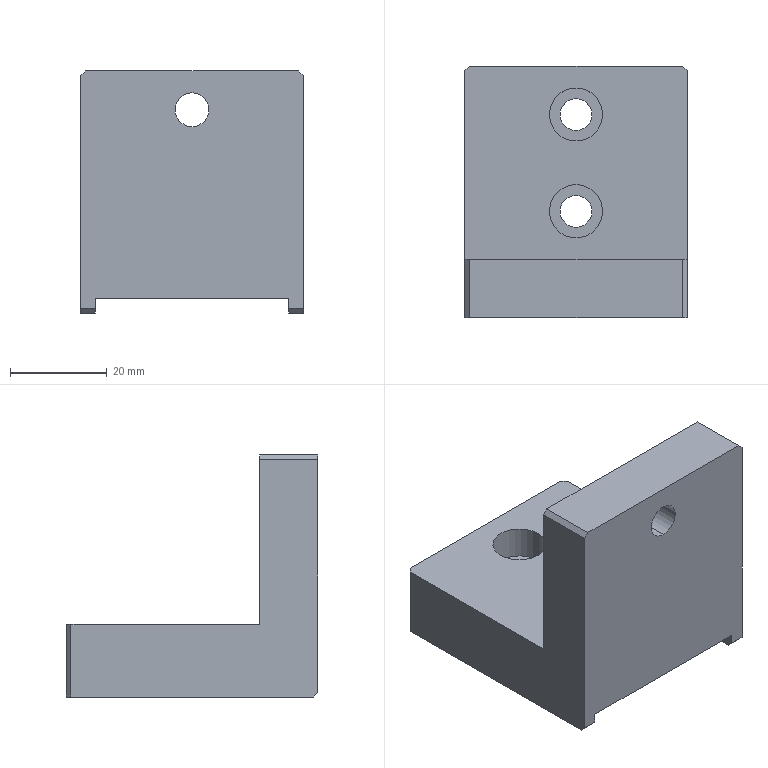Part | SolidWorks | features HoleWzd 2, ICE 2, Chamfer 1, Extrusion 1 | 1 solid | 30 faces | box 46 x 52 x 50 mm | volume 46820 mm3 | plane 20 | cylinder 10 | commonest cylinder face diameters 6.6 x4 11 x4 7 x2
STEP:
#1=CARTESIAN_POINT('',(0.,-6.,13.5));
#2=VERTEX_POINT('',#1);
#3=CARTESIAN_POINT('',(0.,-6.,20.5));
#4=VERTEX_POINT('',#3);
#5=CARTESIAN_POINT('',(0.,-6.,17.));
#6=DIRECTION('',(0.,1.,0.));
#7=DIRECTION('',(0.,0.,1.));
#8=AXIS2_PLACEMENT_3D('',#5,#6,#7);
#9=CIRCLE('',#8,3.5);
#10=EDGE_CURVE('',#2,#4,#9,.T.);
#11=ORIENTED_EDGE('',*,*,#10,.F.);
#12=CARTESIAN_POINT('',(0.,6.,13.5));
#13=VERTEX_POINT('',#12);
#14=CARTESIAN_POINT('',(0.,6.,13.5));
#15=DIRECTION('',(0.,1.,0.));
#16=VECTOR('',#15,1000.);
#17=LINE('',#14,#16);
#18=EDGE_CURVE('',#2,#13,#17,.T.);
#19=ORIENTED_EDGE('',*,*,#18,.T.);
#20=CARTESIAN_POINT('',(0.,6.,20.5));
#21=VERTEX_POINT('',#20);
#22=CARTESIAN_POINT('',(0.,6.,17.));
#23=DIRECTION('',(0.,1.,0.));
#24=DIRECTION('',(0.,0.,1.));
#25=AXIS2_PLACEMENT_3D('',#22,#23,#24);
#26=CIRCLE('',#25,3.5);
#27=EDGE_CURVE('',#13,#21,#26,.T.);
#28=ORIENTED_EDGE('',*,*,#27,.T.);
#29=CARTESIAN_POINT('',(0.,6.,20.5));
#30=DIRECTION('',(0.,1.,0.));
#31=VECTOR('',#30,1000.);
#32=LINE('',#29,#31);
#33=EDGE_CURVE('',#4,#21,#32,.T.);
#34=ORIENTED_EDGE('',*,*,#33,.F.);
#35=EDGE_LOOP('',(#11,#19,#28,#34));
#36=FACE_OUTER_BOUND('',#35,.T.);
#37=CARTESIAN_POINT('',(0.,6.,17.));
#38=DIRECTION('',(0.,1.,0.));
#39=DIRECTION('',(0.,0.,1.));
#40=AXIS2_PLACEMENT_3D('',#37,#38,#39);
#41=CYLINDRICAL_SURFACE('',#40,3.5);
#42=ADVANCED_FACE('',(#36),#41,.F.);
#43=CARTESIAN_POINT('',(-5.5,16.,-16.8));
#44=VERTEX_POINT('',#43);
#45=CARTESIAN_POINT('',(5.5,16.,-16.8));
#46=VERTEX_POINT('',#45);
#47=CARTESIAN_POINT('',(0.,16.,-16.8));
#48=DIRECTION('',(0.,0.,1.));
#49=DIRECTION('',(1.,0.,0.));
#50=AXIS2_PLACEMENT_3D('',#47,#48,#49);
#51=CIRCLE('',#50,5.5);
#52=EDGE_CURVE('',#44,#46,#51,.T.);
#53=ORIENTED_EDGE('',*,*,#52,.F.);
#54=CARTESIAN_POINT('',(-5.5,16.,-10.));
#55=VERTEX_POINT('',#54);
#56=CARTESIAN_POINT('',(-5.5,16.,-10.));
#57=DIRECTION('',(0.,0.,1.));
#58=VECTOR('',#57,1000.);
#59=LINE('',#56,#58);
#60=EDGE_CURVE('',#44,#55,#59,.T.);
#61=ORIENTED_EDGE('',*,*,#60,.T.);
#62=CARTESIAN_POINT('',(5.5,16.,-10.));
#63=VERTEX_POINT('',#62);
#64=CARTESIAN_POINT('',(0.,16.,-10.));
#65=DIRECTION('',(0.,0.,1.));
#66=DIRECTION('',(1.,0.,0.));
#67=AXIS2_PLACEMENT_3D('',#64,#65,#66);
#68=CIRCLE('',#67,5.5);
#69=EDGE_CURVE('',#55,#63,#68,.T.);
#70=ORIENTED_EDGE('',*,*,#69,.T.);
#71=CARTESIAN_POINT('',(5.5,16.,-10.));
#72=DIRECTION('',(0.,0.,1.));
#73=VECTOR('',#72,1000.);
#74=LINE('',#71,#73);
#75=EDGE_CURVE('',#46,#63,#74,.T.);
#76=ORIENTED_EDGE('',*,*,#75,.F.);
#77=EDGE_LOOP('',(#53,#61,#70,#76));
#78=FACE_OUTER_BOUND('',#77,.T.);
#79=CARTESIAN_POINT('',(0.,16.,-10.));
#80=DIRECTION('',(0.,0.,1.));
#81=DIRECTION('',(1.,0.,0.));
#82=AXIS2_PLACEMENT_3D('',#79,#80,#81);
#83=CYLINDRICAL_SURFACE('',#82,5.5);
#84=ADVANCED_FACE('',(#78),#83,.F.);
#85=CARTESIAN_POINT('',(3.3,16.,-22.));
#86=VERTEX_POINT('',#85);
#87=CARTESIAN_POINT('',(-3.3,16.,-22.));
#88=VERTEX_POINT('',#87);
#89=CARTESIAN_POINT('',(0.,16.,-22.));
#90=DIRECTION('',(0.,0.,-1.));
#91=DIRECTION('',(-1.,0.,0.));
#92=AXIS2_PLACEMENT_3D('',#89,#90,#91);
#93=CIRCLE('',#92,3.3);
#94=EDGE_CURVE('',#86,#88,#93,.T.);
#95=ORIENTED_EDGE('',*,*,#94,.T.);
#96=CARTESIAN_POINT('',(-3.3,16.,-16.8));
#97=VERTEX_POINT('',#96);
#98=CARTESIAN_POINT('',(-3.3,16.,-10.));
#99=DIRECTION('',(0.,0.,1.));
#100=VECTOR('',#99,1000.);
#101=LINE('',#98,#100);
#102=EDGE_CURVE('',#88,#97,#101,.T.);
#103=ORIENTED_EDGE('',*,*,#102,.T.);
#104=CARTESIAN_POINT('',(3.3,16.,-16.8));
#105=VERTEX_POINT('',#104);
#106=CARTESIAN_POINT('',(0.,16.,-16.8));
#107=DIRECTION('',(0.,0.,1.));
#108=DIRECTION('',(1.,0.,0.));
#109=AXIS2_PLACEMENT_3D('',#106,#107,#108);
#110=CIRCLE('',#109,3.3);
#111=EDGE_CURVE('',#97,#105,#110,.T.);
#112=ORIENTED_EDGE('',*,*,#111,.T.);
#113=CARTESIAN_POINT('',(3.3,16.,-10.));
#114=DIRECTION('',(0.,0.,1.));
#115=VECTOR('',#114,1000.);
#116=LINE('',#113,#115);
#117=EDGE_CURVE('',#86,#105,#116,.T.);
#118=ORIENTED_EDGE('',*,*,#117,.F.);
#119=EDGE_LOOP('',(#95,#103,#112,#118));
#120=FACE_OUTER_BOUND('',#119,.T.);
#121=CARTESIAN_POINT('',(0.,16.,-10.));
#122=DIRECTION('',(0.,0.,1.));
#123=DIRECTION('',(1.,0.,0.));
#124=AXIS2_PLACEMENT_3D('',#121,#122,#123);
#125=CYLINDRICAL_SURFACE('',#124,3.3);
#126=ADVANCED_FACE('',(#120),#125,.F.);
#127=CARTESIAN_POINT('',(-5.5,36.,-16.8));
#128=VERTEX_POINT('',#127);
#129=CARTESIAN_POINT('',(5.5,36.,-16.8));
#130=VERTEX_POINT('',#129);
#131=CARTESIAN_POINT('',(0.,36.,-16.8));
#132=DIRECTION('',(0.,0.,1.));
#133=DIRECTION('',(1.,0.,0.));
#134=AXIS2_PLACEMENT_3D('',#131,#132,#133);
#135=CIRCLE('',#134,5.5);
#136=EDGE_CURVE('',#128,#130,#135,.T.);
#137=ORIENTED_EDGE('',*,*,#136,.F.);
#138=CARTESIAN_POINT('',(-5.5,36.,-10.));
#139=VERTEX_POINT('',#138);
#140=CARTESIAN_POINT('',(-5.5,36.,-10.));
#141=DIRECTION('',(0.,0.,1.));
#142=VECTOR('',#141,1000.);
#143=LINE('',#140,#142);
#144=EDGE_CURVE('',#128,#139,#143,.T.);
#145=ORIENTED_EDGE('',*,*,#144,.T.);
#146=CARTESIAN_POINT('',(5.5,36.,-10.));
#147=VERTEX_POINT('',#146);
#148=CARTESIAN_POINT('',(0.,36.,-10.));
#149=DIRECTION('',(0.,0.,1.));
#150=DIRECTION('',(1.,0.,0.));
#151=AXIS2_PLACEMENT_3D('',#148,#149,#150);
#152=CIRCLE('',#151,5.5);
#153=EDGE_CURVE('',#139,#147,#152,.T.);
#154=ORIENTED_EDGE('',*,*,#153,.T.);
#155=CARTESIAN_POINT('',(5.5,36.,-10.));
#156=DIRECTION('',(0.,0.,1.));
#157=VECTOR('',#156,1000.);
#158=LINE('',#155,#157);
#159=EDGE_CURVE('',#130,#147,#158,.T.);
#160=ORIENTED_EDGE('',*,*,#159,.F.);
#161=EDGE_LOOP('',(#137,#145,#154,#160));
#162=FACE_OUTER_BOUND('',#161,.T.);
#163=CARTESIAN_POINT('',(0.,36.,-10.));
#164=DIRECTION('',(0.,0.,1.));
#165=DIRECTION('',(1.,0.,0.));
#166=AXIS2_PLACEMENT_3D('',#163,#164,#165);
#167=CYLINDRICAL_SURFACE('',#166,5.5);
#168=ADVANCED_FACE('',(#162),#167,.F.);
#169=CARTESIAN_POINT('',(3.3,36.,-22.));
#170=VERTEX_POINT('',#169);
#171=CARTESIAN_POINT('',(-3.3,36.,-22.));
#172=VERTEX_POINT('',#171);
#173=CARTESIAN_POINT('',(0.,36.,-22.));
#174=DIRECTION('',(0.,0.,-1.));
#175=DIRECTION('',(-1.,0.,0.));
#176=AXIS2_PLACEMENT_3D('',#173,#174,#175);
#177=CIRCLE('',#176,3.3);
#178=EDGE_CURVE('',#170,#172,#177,.T.);
#179=ORIENTED_EDGE('',*,*,#178,.T.);
#180=CARTESIAN_POINT('',(-3.3,36.,-16.8));
#181=VERTEX_POINT('',#180);
#182=CARTESIAN_POINT('',(-3.3,36.,-10.));
#183=DIRECTION('',(0.,0.,1.));
#184=VECTOR('',#183,1000.);
#185=LINE('',#182,#184);
#186=EDGE_CURVE('',#172,#181,#185,.T.);
#187=ORIENTED_EDGE('',*,*,#186,.T.);
#188=CARTESIAN_POINT('',(3.3,36.,-16.8));
#189=VERTEX_POINT('',#188);
#190=CARTESIAN_POINT('',(0.,36.,-16.8));
#191=DIRECTION('',(0.,0.,1.));
#192=DIRECTION('',(1.,0.,0.));
#193=AXIS2_PLACEMENT_3D('',#190,#191,#192);
#194=CIRCLE('',#193,3.3);
#195=EDGE_CURVE('',#181,#189,#194,.T.);
#196=ORIENTED_EDGE('',*,*,#195,.T.);
#197=CARTESIAN_POINT('',(3.3,36.,-10.));
#198=DIRECTION('',(0.,0.,1.));
#199=VECTOR('',#198,1000.);
#200=LINE('',#197,#199);
#201=EDGE_CURVE('',#170,#189,#200,.T.);
#202=ORIENTED_EDGE('',*,*,#201,.F.);
#203=EDGE_LOOP('',(#179,#187,#196,#202));
#204=FACE_OUTER_BOUND('',#203,.T.);
#205=CARTESIAN_POINT('',(0.,36.,-10.));
#206=DIRECTION('',(0.,0.,1.));
#207=DIRECTION('',(1.,0.,0.));
#208=AXIS2_PLACEMENT_3D('',#205,#206,#207);
#209=CYLINDRICAL_SURFACE('',#208,3.3);
#210=ADVANCED_FACE('',(#204),#209,.F.);
#211=CARTESIAN_POINT('',(-22.,6.,25.));
#212=VERTEX_POINT('',#211);
#213=CARTESIAN_POINT('',(22.,6.,25.));
#214=VERTEX_POINT('',#213);
#215=CARTESIAN_POINT('',(-23.,6.,25.));
#216=DIRECTION('',(1.,0.,0.));
#217=VECTOR('',#216,1000.);
#218=LINE('',#215,#217);
#219=EDGE_CURVE('',#212,#214,#218,.T.);
#220=ORIENTED_EDGE('',*,*,#219,.T.);
#221=CARTESIAN_POINT('',(23.,6.,24.));
#222=VERTEX_POINT('',#221);
#223=CARTESIAN_POINT('',(23.,6.,24.));
#224=DIRECTION('',(0.7071,0.,-0.7071));
#225=VECTOR('',#224,1000.);
#226=LINE('',#223,#225);
#227=EDGE_CURVE('',#214,#222,#226,.T.);
#228=ORIENTED_EDGE('',*,*,#227,.T.);
#229=CARTESIAN_POINT('',(23.,6.,-10.));
#230=VERTEX_POINT('',#229);
#231=CARTESIAN_POINT('',(23.,6.,25.));
#232=DIRECTION('',(0.,0.,-1.));
#233=VECTOR('',#232,1000.);
#234=LINE('',#231,#233);
#235=EDGE_CURVE('',#222,#230,#234,.T.);
#236=ORIENTED_EDGE('',*,*,#235,.T.);
#237=CARTESIAN_POINT('',(-23.,6.,-10.));
#238=VERTEX_POINT('',#237);
#239=CARTESIAN_POINT('',(23.,6.,-10.));
#240=DIRECTION('',(1.,0.,0.));
#241=VECTOR('',#240,1000.);
#242=LINE('',#239,#241);
#243=EDGE_CURVE('',#238,#230,#242,.T.);
#244=ORIENTED_EDGE('',*,*,#243,.F.);
#245=CARTESIAN_POINT('',(-23.,6.,24.));
#246=VERTEX_POINT('',#245);
#247=CARTESIAN_POINT('',(-23.,6.,25.));
#248=DIRECTION('',(0.,0.,1.));
#249=VECTOR('',#248,1000.);
#250=LINE('',#247,#249);
#251=EDGE_CURVE('',#238,#246,#250,.T.);
#252=ORIENTED_EDGE('',*,*,#251,.T.);
#253=CARTESIAN_POINT('',(-22.,6.,25.));
#254=DIRECTION('',(0.7071,0.,0.7071));
#255=VECTOR('',#254,1000.);
#256=LINE('',#253,#255);
#257=EDGE_CURVE('',#246,#212,#256,.T.);
#258=ORIENTED_EDGE('',*,*,#257,.T.);
#259=EDGE_LOOP('',(#220,#228,#236,#244,#252,#258));
#260=FACE_OUTER_BOUND('',#259,.T.);
#261=CARTESIAN_POINT('',(0.,6.,17.));
#262=DIRECTION('',(0.,1.,0.));
#263=DIRECTION('',(0.,0.,1.));
#264=AXIS2_PLACEMENT_3D('',#261,#262,#263);
#265=CIRCLE('',#264,3.5);
#266=EDGE_CURVE('',#21,#13,#265,.T.);
#267=ORIENTED_EDGE('',*,*,#266,.F.);
#268=ORIENTED_EDGE('',*,*,#27,.F.);
#269=EDGE_LOOP('',(#267,#268));
#270=FACE_BOUND('',#269,.T.);
#271=CARTESIAN_POINT('',(0.,6.,0.));
#272=DIRECTION('',(0.,-1.,0.));
#273=DIRECTION('',(0.,0.,-1.));
#274=AXIS2_PLACEMENT_3D('',#271,#272,#273);
#275=PLANE('',#274);
#276=ADVANCED_FACE('',(#260,#270),#275,.F.);
#277=CARTESIAN_POINT('',(23.,45.,-25.));
#278=VERTEX_POINT('',#277);
#279=CARTESIAN_POINT('',(23.,-5.,-25.));
#280=VERTEX_POINT('',#279);
#281=CARTESIAN_POINT('',(23.,6.,-25.));
#282=DIRECTION('',(0.,-1.,0.));
#283=VECTOR('',#282,1000.);
#284=LINE('',#281,#283);
#285=EDGE_CURVE('',#278,#280,#284,.T.);
#286=ORIENTED_EDGE('',*,*,#285,.T.);
#287=CARTESIAN_POINT('',(20.,-5.,-25.));
#288=VERTEX_POINT('',#287);
#289=CARTESIAN_POINT('',(20.,-5.,-25.));
#290=DIRECTION('',(-1.,0.,0.));
#291=VECTOR('',#290,1000.);
#292=LINE('',#289,#291);
#293=EDGE_CURVE('',#280,#288,#292,.T.);
#294=ORIENTED_EDGE('',*,*,#293,.T.);
#295=CARTESIAN_POINT('',(20.,46.,-25.));
#296=VERTEX_POINT('',#295);
#297=CARTESIAN_POINT('',(20.,46.,-25.));
#298=DIRECTION('',(0.,-1.,0.));
#299=VECTOR('',#298,1000.);
#300=LINE('',#297,#299);
#301=EDGE_CURVE('',#296,#288,#300,.T.);
#302=ORIENTED_EDGE('',*,*,#301,.F.);
#303=CARTESIAN_POINT('',(22.,46.,-25.));
#304=VERTEX_POINT('',#303);
#305=CARTESIAN_POINT('',(23.,46.,-25.));
#306=DIRECTION('',(-1.,0.,0.));
#307=VECTOR('',#306,1000.);
#308=LINE('',#305,#307);
#309=EDGE_CURVE('',#304,#296,#308,.T.);
#310=ORIENTED_EDGE('',*,*,#309,.F.);
#311=CARTESIAN_POINT('',(22.,46.,-25.));
#312=DIRECTION('',(0.7071,-0.7071,0.));
#313=VECTOR('',#312,1000.);
#314=LINE('',#311,#313);
#315=EDGE_CURVE('',#304,#278,#314,.T.);
#316=ORIENTED_EDGE('',*,*,#315,.T.);
#317=EDGE_LOOP('',(#286,#294,#302,#310,#316));
#318=FACE_OUTER_BOUND('',#317,.T.);
#319=CARTESIAN_POINT('',(-23.,6.,-25.));
#320=DIRECTION('',(0.,0.,1.));
#321=DIRECTION('',(1.,0.,0.));
#322=AXIS2_PLACEMENT_3D('',#319,#320,#321);
#323=PLANE('',#322);
#324=ADVANCED_FACE('',(#318),#323,.F.);
#325=CARTESIAN_POINT('',(23.,-6.,24.));
#326=VERTEX_POINT('',#325);
#327=CARTESIAN_POINT('',(23.,-6.,-24.));
#328=VERTEX_POINT('',#327);
#329=CARTESIAN_POINT('',(23.,-6.,25.));
#330=DIRECTION('',(0.,0.,-1.));
#331=VECTOR('',#330,1000.);
#332=LINE('',#329,#331);
#333=EDGE_CURVE('',#326,#328,#332,.T.);
#334=ORIENTED_EDGE('',*,*,#333,.T.);
#335=CARTESIAN_POINT('',(23.,-5.,-25.));
#336=DIRECTION('',(0.,0.7071,-0.7071));
#337=VECTOR('',#336,1000.);
#338=LINE('',#335,#337);
#339=EDGE_CURVE('',#328,#280,#338,.T.);
#340=ORIENTED_EDGE('',*,*,#339,.T.);
#341=ORIENTED_EDGE('',*,*,#285,.F.);
#342=CARTESIAN_POINT('',(23.,45.,-10.));
#343=VERTEX_POINT('',#342);
#344=CARTESIAN_POINT('',(23.,45.,25.));
#345=DIRECTION('',(0.,0.,1.));
#346=VECTOR('',#345,1000.);
#347=LINE('',#344,#346);
#348=EDGE_CURVE('',#278,#343,#347,.T.);
#349=ORIENTED_EDGE('',*,*,#348,.T.);
#350=CARTESIAN_POINT('',(23.,46.,-10.));
#351=DIRECTION('',(0.,-1.,0.));
#352=VECTOR('',#351,1000.);
#353=LINE('',#350,#352);
#354=EDGE_CURVE('',#343,#230,#353,.T.);
#355=ORIENTED_EDGE('',*,*,#354,.T.);
#356=ORIENTED_EDGE('',*,*,#235,.F.);
#357=CARTESIAN_POINT('',(23.,6.,24.));
#358=DIRECTION('',(0.,-1.,0.));
#359=VECTOR('',#358,1000.);
#360=LINE('',#357,#359);
#361=EDGE_CURVE('',#222,#326,#360,.T.);
#362=ORIENTED_EDGE('',*,*,#361,.T.);
#363=EDGE_LOOP('',(#334,#340,#341,#349,#355,#356,#362));
#364=FACE_OUTER_BOUND('',#363,.T.);
#365=CARTESIAN_POINT('',(23.,6.,25.));
#366=DIRECTION('',(-1.,0.,0.));
#367=DIRECTION('',(0.,0.,1.));
#368=AXIS2_PLACEMENT_3D('',#365,#366,#367);
#369=PLANE('',#368);
#370=ADVANCED_FACE('',(#364),#369,.F.);
#371=CARTESIAN_POINT('',(-20.,-5.,-25.));
#372=VERTEX_POINT('',#371);
#373=CARTESIAN_POINT('',(-20.,46.,-25.));
#374=VERTEX_POINT('',#373);
#375=CARTESIAN_POINT('',(-20.,46.,-25.));
#376=DIRECTION('',(0.,1.,0.));
#377=VECTOR('',#376,1000.);
#378=LINE('',#375,#377);
#379=EDGE_CURVE('',#372,#374,#378,.T.);
#380=ORIENTED_EDGE('',*,*,#379,.F.);
#381=CARTESIAN_POINT('',(-23.,-5.,-25.));
#382=VERTEX_POINT('',#381);
#383=CARTESIAN_POINT('',(-23.,-5.,-25.));
#384=DIRECTION('',(-1.,0.,0.));
#385=VECTOR('',#384,1000.);
#386=LINE('',#383,#385);
#387=EDGE_CURVE('',#372,#382,#386,.T.);
#388=ORIENTED_EDGE('',*,*,#387,.T.);
#389=CARTESIAN_POINT('',(-23.,45.,-25.));
#390=VERTEX_POINT('',#389);
#391=CARTESIAN_POINT('',(-23.,6.,-25.));
#392=DIRECTION('',(0.,-1.,0.));
#393=VECTOR('',#392,1000.);
#394=LINE('',#391,#393);
#395=EDGE_CURVE('',#390,#382,#394,.T.);
#396=ORIENTED_EDGE('',*,*,#395,.F.);
#397=CARTESIAN_POINT('',(-22.,46.,-25.));
#398=VERTEX_POINT('',#397);
#399=CARTESIAN_POINT('',(-22.,46.,-25.));
#400=DIRECTION('',(0.7071,0.7071,0.));
#401=VECTOR('',#400,1000.);
#402=LINE('',#399,#401);
#403=EDGE_CURVE('',#390,#398,#402,.T.);
#404=ORIENTED_EDGE('',*,*,#403,.T.);
#405=CARTESIAN_POINT('',(23.,46.,-25.));
#406=DIRECTION('',(-1.,0.,0.));
#407=VECTOR('',#406,1000.);
#408=LINE('',#405,#407);
#409=EDGE_CURVE('',#374,#398,#408,.T.);
#410=ORIENTED_EDGE('',*,*,#409,.F.);
#411=EDGE_LOOP('',(#380,#388,#396,#404,#410));
#412=FACE_OUTER_BOUND('',#411,.T.);
#413=CARTESIAN_POINT('',(-23.,6.,-25.));
#414=DIRECTION('',(0.,0.,1.));
#415=DIRECTION('',(1.,0.,0.));
#416=AXIS2_PLACEMENT_3D('',#413,#414,#415);
#417=PLANE('',#416);
#418=ADVANCED_FACE('',(#412),#417,.F.);
#419=ORIENTED_EDGE('',*,*,#395,.T.);
#420=CARTESIAN_POINT('',(-23.,-6.,-24.));
#421=VERTEX_POINT('',#420);
#422=CARTESIAN_POINT('',(-23.,-5.,-25.));
#423=DIRECTION('',(0.,-0.7071,0.7071));
#424=VECTOR('',#423,1000.);
#425=LINE('',#422,#424);
#426=EDGE_CURVE('',#382,#421,#425,.T.);
#427=ORIENTED_EDGE('',*,*,#426,.T.);
#428=CARTESIAN_POINT('',(-23.,-6.,24.));
#429=VERTEX_POINT('',#428);
#430=CARTESIAN_POINT('',(-23.,-6.,25.));
#431=DIRECTION('',(0.,0.,1.));
#432=VECTOR('',#431,1000.);
#433=LINE('',#430,#432);
#434=EDGE_CURVE('',#421,#429,#433,.T.);
#435=ORIENTED_EDGE('',*,*,#434,.T.);
#436=CARTESIAN_POINT('',(-23.,6.,24.));
#437=DIRECTION('',(0.,1.,0.));
#438=VECTOR('',#437,1000.);
#439=LINE('',#436,#438);
#440=EDGE_CURVE('',#429,#246,#439,.T.);
#441=ORIENTED_EDGE('',*,*,#440,.T.);
#442=ORIENTED_EDGE('',*,*,#251,.F.);
#443=CARTESIAN_POINT('',(-23.,45.,-10.));
#444=VERTEX_POINT('',#443);
#445=CARTESIAN_POINT('',(-23.,46.,-10.));
#446=DIRECTION('',(0.,-1.,0.));
#447=VECTOR('',#446,1000.);
#448=LINE('',#445,#447);
#449=EDGE_CURVE('',#444,#238,#448,.T.);
#450=ORIENTED_EDGE('',*,*,#449,.F.);
#451=CARTESIAN_POINT('',(-23.,45.,25.));
#452=DIRECTION('',(0.,0.,-1.));
#453=VECTOR('',#452,1000.);
#454=LINE('',#451,#453);
#455=EDGE_CURVE('',#444,#390,#454,.T.);
#456=ORIENTED_EDGE('',*,*,#455,.T.);
#457=EDGE_LOOP('',(#419,#427,#435,#441,#442,#450,#456));
#458=FACE_OUTER_BOUND('',#457,.T.);
#459=CARTESIAN_POINT('',(-23.,6.,25.));
#460=DIRECTION('',(1.,0.,0.));
#461=DIRECTION('',(0.,0.,-1.));
#462=AXIS2_PLACEMENT_3D('',#459,#460,#461);
#463=PLANE('',#462);
#464=ADVANCED_FACE('',(#458),#463,.F.);
#465=CARTESIAN_POINT('',(-22.,-6.,25.));
#466=VERTEX_POINT('',#465);
#467=CARTESIAN_POINT('',(22.,-6.,25.));
#468=VERTEX_POINT('',#467);
#469=CARTESIAN_POINT('',(-23.,-6.,25.));
#470=DIRECTION('',(1.,0.,0.));
#471=VECTOR('',#470,1000.);
#472=LINE('',#469,#471);
#473=EDGE_CURVE('',#466,#468,#472,.T.);
#474=ORIENTED_EDGE('',*,*,#473,.T.);
#475=CARTESIAN_POINT('',(22.,6.,25.));
#476=DIRECTION('',(0.,1.,0.));
#477=VECTOR('',#476,1000.);
#478=LINE('',#475,#477);
#479=EDGE_CURVE('',#468,#214,#478,.T.);
#480=ORIENTED_EDGE('',*,*,#479,.T.);
#481=ORIENTED_EDGE('',*,*,#219,.F.);
#482=CARTESIAN_POINT('',(-22.,6.,25.));
#483=DIRECTION('',(0.,-1.,0.));
#484=VECTOR('',#483,1000.);
#485=LINE('',#482,#484);
#486=EDGE_CURVE('',#212,#466,#485,.T.);
#487=ORIENTED_EDGE('',*,*,#486,.T.);
#488=EDGE_LOOP('',(#474,#480,#481,#487));
#489=FACE_OUTER_BOUND('',#488,.T.);
#490=CARTESIAN_POINT('',(-23.,6.,25.));
#491=DIRECTION('',(0.,0.,-1.));
#492=DIRECTION('',(-1.,0.,0.));
#493=AXIS2_PLACEMENT_3D('',#490,#491,#492);
#494=PLANE('',#493);
#495=ADVANCED_FACE('',(#489),#494,.F.);
#496=CARTESIAN_POINT('',(0.,-6.,17.));
#497=DIRECTION('',(0.,1.,0.));
#498=DIRECTION('',(0.,0.,1.));
#499=AXIS2_PLACEMENT_3D('',#496,#497,#498);
#500=CIRCLE('',#499,3.5);
#501=EDGE_CURVE('',#4,#2,#500,.T.);
#502=ORIENTED_EDGE('',*,*,#501,.T.);
#503=ORIENTED_EDGE('',*,*,#10,.T.);
#504=EDGE_LOOP('',(#502,#503));
#505=FACE_BOUND('',#504,.T.);
#506=CARTESIAN_POINT('',(20.,-6.,-22.));
#507=VERTEX_POINT('',#506);
#508=CARTESIAN_POINT('',(20.,-6.,-24.));
#509=VERTEX_POINT('',#508);
#510=CARTESIAN_POINT('',(20.,-6.,-22.));
#511=DIRECTION('',(0.,0.,-1.));
#512=VECTOR('',#511,1000.);
#513=LINE('',#510,#512);
#514=EDGE_CURVE('',#507,#509,#513,.T.);
#515=ORIENTED_EDGE('',*,*,#514,.T.);
#516=CARTESIAN_POINT('',(23.,-6.,-24.));
#517=DIRECTION('',(1.,0.,0.));
#518=VECTOR('',#517,1000.);
#519=LINE('',#516,#518);
#520=EDGE_CURVE('',#509,#328,#519,.T.);
#521=ORIENTED_EDGE('',*,*,#520,.T.);
#522=ORIENTED_EDGE('',*,*,#333,.F.);
#523=CARTESIAN_POINT('',(23.5,-6.,23.5));
#524=DIRECTION('',(-0.7071,0.,0.7071));
#525=VECTOR('',#524,1000.);
#526=LINE('',#523,#525);
#527=EDGE_CURVE('',#326,#468,#526,.T.);
#528=ORIENTED_EDGE('',*,*,#527,.T.);
#529=ORIENTED_EDGE('',*,*,#473,.F.);
#530=CARTESIAN_POINT('',(-23.5,-6.,23.5));
#531=DIRECTION('',(-0.7071,0.,-0.7071));
#532=VECTOR('',#531,1000.);
#533=LINE('',#530,#532);
#534=EDGE_CURVE('',#466,#429,#533,.T.);
#535=ORIENTED_EDGE('',*,*,#534,.T.);
#536=ORIENTED_EDGE('',*,*,#434,.F.);
#537=CARTESIAN_POINT('',(-20.,-6.,-24.));
#538=VERTEX_POINT('',#537);
#539=CARTESIAN_POINT('',(-20.,-6.,-24.));
#540=DIRECTION('',(1.,0.,0.));
#541=VECTOR('',#540,1000.);
#542=LINE('',#539,#541);
#543=EDGE_CURVE('',#421,#538,#542,.T.);
#544=ORIENTED_EDGE('',*,*,#543,.T.);
#545=CARTESIAN_POINT('',(-20.,-6.,-22.));
#546=VERTEX_POINT('',#545);
#547=CARTESIAN_POINT('',(-20.,-6.,-22.));
#548=DIRECTION('',(0.,0.,-1.));
#549=VECTOR('',#548,1000.);
#550=LINE('',#547,#549);
#551=EDGE_CURVE('',#546,#538,#550,.T.);
#552=ORIENTED_EDGE('',*,*,#551,.F.);
#553=CARTESIAN_POINT('',(20.,-6.,-22.));
#554=DIRECTION('',(-1.,0.,0.));
#555=VECTOR('',#554,1000.);
#556=LINE('',#553,#555);
#557=EDGE_CURVE('',#507,#546,#556,.T.);
#558=ORIENTED_EDGE('',*,*,#557,.F.);
#559=EDGE_LOOP('',(#515,#521,#522,#528,#529,#535,#536,#544,#552,#558));
#560=FACE_OUTER_BOUND('',#559,.T.);
#561=CARTESIAN_POINT('',(0.,-6.,0.));
#562=DIRECTION('',(0.,-1.,0.));
#563=DIRECTION('',(0.,0.,-1.));
#564=AXIS2_PLACEMENT_3D('',#561,#562,#563);
#565=PLANE('',#564);
#566=ADVANCED_FACE('',(#505,#560),#565,.T.);
#567=CARTESIAN_POINT('',(0.,16.,-10.));
#568=DIRECTION('',(0.,0.,1.));
#569=DIRECTION('',(1.,0.,0.));
#570=AXIS2_PLACEMENT_3D('',#567,#568,#569);
#571=CIRCLE('',#570,5.5);
#572=EDGE_CURVE('',#63,#55,#571,.T.);
#573=ORIENTED_EDGE('',*,*,#572,.F.);
#574=ORIENTED_EDGE('',*,*,#69,.F.);
#575=EDGE_LOOP('',(#573,#574));
#576=FACE_BOUND('',#575,.T.);
#577=CARTESIAN_POINT('',(0.,36.,-10.));
#578=DIRECTION('',(0.,0.,1.));
#579=DIRECTION('',(1.,0.,0.));
#580=AXIS2_PLACEMENT_3D('',#577,#578,#579);
#581=CIRCLE('',#580,5.5);
#582=EDGE_CURVE('',#147,#139,#581,.T.);
#583=ORIENTED_EDGE('',*,*,#582,.F.);
#584=ORIENTED_EDGE('',*,*,#153,.F.);
#585=EDGE_LOOP('',(#583,#584));
#586=FACE_BOUND('',#585,.T.);
#587=CARTESIAN_POINT('',(-22.,46.,-10.));
#588=VERTEX_POINT('',#587);
#589=CARTESIAN_POINT('',(22.,46.,-10.));
#590=VERTEX_POINT('',#589);
#591=CARTESIAN_POINT('',(23.,46.,-10.));
#592=DIRECTION('',(1.,0.,0.));
#593=VECTOR('',#592,1000.);
#594=LINE('',#591,#593);
#595=EDGE_CURVE('',#588,#590,#594,.T.);
#596=ORIENTED_EDGE('',*,*,#595,.F.);
#597=CARTESIAN_POINT('',(-22.,46.,-10.));
#598=DIRECTION('',(-0.7071,-0.7071,0.));
#599=VECTOR('',#598,1000.);
#600=LINE('',#597,#599);
#601=EDGE_CURVE('',#588,#444,#600,.T.);
#602=ORIENTED_EDGE('',*,*,#601,.T.);
#603=ORIENTED_EDGE('',*,*,#449,.T.);
#604=ORIENTED_EDGE('',*,*,#243,.T.);
#605=ORIENTED_EDGE('',*,*,#354,.F.);
#606=CARTESIAN_POINT('',(22.,46.,-10.));
#607=DIRECTION('',(-0.7071,0.7071,0.));
#608=VECTOR('',#607,1000.);
#609=LINE('',#606,#608);
#610=EDGE_CURVE('',#343,#590,#609,.T.);
#611=ORIENTED_EDGE('',*,*,#610,.T.);
#612=EDGE_LOOP('',(#596,#602,#603,#604,#605,#611));
#613=FACE_OUTER_BOUND('',#612,.T.);
#614=CARTESIAN_POINT('',(23.,46.,-10.));
#615=DIRECTION('',(0.,0.,-1.));
#616=DIRECTION('',(-1.,0.,0.));
#617=AXIS2_PLACEMENT_3D('',#614,#615,#616);
#618=PLANE('',#617);
#619=ADVANCED_FACE('',(#576,#586,#613),#618,.F.);
#620=ORIENTED_EDGE('',*,*,#409,.T.);
#621=CARTESIAN_POINT('',(-22.,46.,0.));
#622=DIRECTION('',(0.,0.,1.));
#623=VECTOR('',#622,1000.);
#624=LINE('',#621,#623);
#625=EDGE_CURVE('',#398,#588,#624,.T.);
#626=ORIENTED_EDGE('',*,*,#625,.T.);
#627=ORIENTED_EDGE('',*,*,#595,.T.);
#628=CARTESIAN_POINT('',(22.,46.,0.));
#629=DIRECTION('',(0.,0.,-1.));
#630=VECTOR('',#629,1000.);
#631=LINE('',#628,#630);
#632=EDGE_CURVE('',#590,#304,#631,.T.);
#633=ORIENTED_EDGE('',*,*,#632,.T.);
#634=ORIENTED_EDGE('',*,*,#309,.T.);
#635=CARTESIAN_POINT('',(20.,46.,-22.));
#636=VERTEX_POINT('',#635);
#637=CARTESIAN_POINT('',(20.,46.,-22.));
#638=DIRECTION('',(0.,0.,-1.));
#639=VECTOR('',#638,1000.);
#640=LINE('',#637,#639);
#641=EDGE_CURVE('',#636,#296,#640,.T.);
#642=ORIENTED_EDGE('',*,*,#641,.F.);
#643=CARTESIAN_POINT('',(-20.,46.,-22.));
#644=VERTEX_POINT('',#643);
#645=CARTESIAN_POINT('',(20.,46.,-22.));
#646=DIRECTION('',(1.,0.,0.));
#647=VECTOR('',#646,1000.);
#648=LINE('',#645,#647);
#649=EDGE_CURVE('',#644,#636,#648,.T.);
#650=ORIENTED_EDGE('',*,*,#649,.F.);
#651=CARTESIAN_POINT('',(-20.,46.,-22.));
#652=DIRECTION('',(0.,0.,-1.));
#653=VECTOR('',#652,1000.);
#654=LINE('',#651,#653);
#655=EDGE_CURVE('',#644,#374,#654,.T.);
#656=ORIENTED_EDGE('',*,*,#655,.T.);
#657=EDGE_LOOP('',(#620,#626,#627,#633,#634,#642,#650,#656));
#658=FACE_OUTER_BOUND('',#657,.T.);
#659=CARTESIAN_POINT('',(0.,46.,0.));
#660=DIRECTION('',(0.,-1.,0.));
#661=DIRECTION('',(0.,0.,-1.));
#662=AXIS2_PLACEMENT_3D('',#659,#660,#661);
#663=PLANE('',#662);
#664=ADVANCED_FACE('',(#658),#663,.F.);
#665=ORIENTED_EDGE('',*,*,#301,.T.);
#666=CARTESIAN_POINT('',(20.,-5.,-25.));
#667=DIRECTION('',(0.,-0.7071,0.7071));
#668=VECTOR('',#667,1000.);
#669=LINE('',#666,#668);
#670=EDGE_CURVE('',#288,#509,#669,.T.);
#671=ORIENTED_EDGE('',*,*,#670,.T.);
#672=ORIENTED_EDGE('',*,*,#514,.F.);
#673=CARTESIAN_POINT('',(20.,46.,-22.));
#674=DIRECTION('',(0.,-1.,0.));
#675=VECTOR('',#674,1000.);
#676=LINE('',#673,#675);
#677=EDGE_CURVE('',#636,#507,#676,.T.);
#678=ORIENTED_EDGE('',*,*,#677,.F.);
#679=ORIENTED_EDGE('',*,*,#641,.T.);
#680=EDGE_LOOP('',(#665,#671,#672,#678,#679));
#681=FACE_OUTER_BOUND('',#680,.T.);
#682=CARTESIAN_POINT('',(20.,46.,-22.));
#683=DIRECTION('',(1.,0.,0.));
#684=DIRECTION('',(0.,1.,0.));
#685=AXIS2_PLACEMENT_3D('',#682,#683,#684);
#686=PLANE('',#685);
#687=ADVANCED_FACE('',(#681),#686,.F.);
#688=ORIENTED_EDGE('',*,*,#551,.T.);
#689=CARTESIAN_POINT('',(-20.,-5.,-25.));
#690=DIRECTION('',(0.,0.7071,-0.7071));
#691=VECTOR('',#690,1000.);
#692=LINE('',#689,#691);
#693=EDGE_CURVE('',#538,#372,#692,.T.);
#694=ORIENTED_EDGE('',*,*,#693,.T.);
#695=ORIENTED_EDGE('',*,*,#379,.T.);
#696=ORIENTED_EDGE('',*,*,#655,.F.);
#697=CARTESIAN_POINT('',(-20.,46.,-22.));
#698=DIRECTION('',(0.,1.,0.));
#699=VECTOR('',#698,1000.);
#700=LINE('',#697,#699);
#701=EDGE_CURVE('',#546,#644,#700,.T.);
#702=ORIENTED_EDGE('',*,*,#701,.F.);
#703=EDGE_LOOP('',(#688,#694,#695,#696,#702));
#704=FACE_OUTER_BOUND('',#703,.T.);
#705=CARTESIAN_POINT('',(-20.,46.,-22.));
#706=DIRECTION('',(-1.,0.,0.));
#707=DIRECTION('',(0.,-1.,0.));
#708=AXIS2_PLACEMENT_3D('',#705,#706,#707);
#709=PLANE('',#708);
#710=ADVANCED_FACE('',(#704),#709,.F.);
#711=ORIENTED_EDGE('',*,*,#94,.F.);
#712=CARTESIAN_POINT('',(0.,16.,-22.));
#713=DIRECTION('',(0.,0.,-1.));
#714=DIRECTION('',(-1.,0.,0.));
#715=AXIS2_PLACEMENT_3D('',#712,#713,#714);
#716=CIRCLE('',#715,3.3);
#717=EDGE_CURVE('',#88,#86,#716,.T.);
#718=ORIENTED_EDGE('',*,*,#717,.F.);
#719=EDGE_LOOP('',(#711,#718));
#720=FACE_BOUND('',#719,.T.);
#721=ORIENTED_EDGE('',*,*,#178,.F.);
#722=CARTESIAN_POINT('',(0.,36.,-22.));
#723=DIRECTION('',(0.,0.,-1.));
#724=DIRECTION('',(-1.,0.,0.));
#725=AXIS2_PLACEMENT_3D('',#722,#723,#724);
#726=CIRCLE('',#725,3.3);
#727=EDGE_CURVE('',#172,#170,#726,.T.);
#728=ORIENTED_EDGE('',*,*,#727,.F.);
#729=EDGE_LOOP('',(#721,#728));
#730=FACE_BOUND('',#729,.T.);
#731=ORIENTED_EDGE('',*,*,#677,.T.);
#732=ORIENTED_EDGE('',*,*,#557,.T.);
#733=ORIENTED_EDGE('',*,*,#701,.T.);
#734=ORIENTED_EDGE('',*,*,#649,.T.);
#735=EDGE_LOOP('',(#731,#732,#733,#734));
#736=FACE_OUTER_BOUND('',#735,.T.);
#737=CARTESIAN_POINT('',(0.,0.,-22.));
#738=DIRECTION('',(0.,0.,-1.));
#739=DIRECTION('',(-1.,0.,0.));
#740=AXIS2_PLACEMENT_3D('',#737,#738,#739);
#741=PLANE('',#740);
#742=ADVANCED_FACE('',(#720,#730,#736),#741,.T.);
#743=ORIENTED_EDGE('',*,*,#339,.F.);
#744=ORIENTED_EDGE('',*,*,#520,.F.);
#745=ORIENTED_EDGE('',*,*,#670,.F.);
#746=ORIENTED_EDGE('',*,*,#293,.F.);
#747=EDGE_LOOP('',(#743,#744,#745,#746));
#748=FACE_OUTER_BOUND('',#747,.T.);
#749=CARTESIAN_POINT('',(-23.,-5.,-25.));
#750=DIRECTION('',(0.,-0.7071,-0.7071));
#751=DIRECTION('',(1.,0.,0.));
#752=AXIS2_PLACEMENT_3D('',#749,#750,#751);
#753=PLANE('',#752);
#754=ADVANCED_FACE('',(#748),#753,.T.);
#755=ORIENTED_EDGE('',*,*,#693,.F.);
#756=ORIENTED_EDGE('',*,*,#543,.F.);
#757=ORIENTED_EDGE('',*,*,#426,.F.);
#758=ORIENTED_EDGE('',*,*,#387,.F.);
#759=EDGE_LOOP('',(#755,#756,#757,#758));
#760=FACE_OUTER_BOUND('',#759,.T.);
#761=CARTESIAN_POINT('',(-23.,-5.,-25.));
#762=DIRECTION('',(0.,-0.7071,-0.7071));
#763=DIRECTION('',(1.,0.,0.));
#764=AXIS2_PLACEMENT_3D('',#761,#762,#763);
#765=PLANE('',#764);
#766=ADVANCED_FACE('',(#760),#765,.T.);
#767=ORIENTED_EDGE('',*,*,#227,.F.);
#768=ORIENTED_EDGE('',*,*,#479,.F.);
#769=ORIENTED_EDGE('',*,*,#527,.F.);
#770=ORIENTED_EDGE('',*,*,#361,.F.);
#771=EDGE_LOOP('',(#767,#768,#769,#770));
#772=FACE_OUTER_BOUND('',#771,.T.);
#773=CARTESIAN_POINT('',(23.,6.,24.));
#774=DIRECTION('',(-0.7071,0.,-0.7071));
#775=DIRECTION('',(0.,-1.,0.));
#776=AXIS2_PLACEMENT_3D('',#773,#774,#775);
#777=PLANE('',#776);
#778=ADVANCED_FACE('',(#772),#777,.F.);
#779=ORIENTED_EDGE('',*,*,#257,.F.);
#780=ORIENTED_EDGE('',*,*,#440,.F.);
#781=ORIENTED_EDGE('',*,*,#534,.F.);
#782=ORIENTED_EDGE('',*,*,#486,.F.);
#783=EDGE_LOOP('',(#779,#780,#781,#782));
#784=FACE_OUTER_BOUND('',#783,.T.);
#785=CARTESIAN_POINT('',(-22.,6.,25.));
#786=DIRECTION('',(0.7071,0.,-0.7071));
#787=DIRECTION('',(0.,-1.,0.));
#788=AXIS2_PLACEMENT_3D('',#785,#786,#787);
#789=PLANE('',#788);
#790=ADVANCED_FACE('',(#784),#789,.F.);
#791=ORIENTED_EDGE('',*,*,#403,.F.);
#792=ORIENTED_EDGE('',*,*,#455,.F.);
#793=ORIENTED_EDGE('',*,*,#601,.F.);
#794=ORIENTED_EDGE('',*,*,#625,.F.);
#795=EDGE_LOOP('',(#791,#792,#793,#794));
#796=FACE_OUTER_BOUND('',#795,.T.);
#797=CARTESIAN_POINT('',(-22.,46.,0.));
#798=DIRECTION('',(0.7071,-0.7071,0.));
#799=DIRECTION('',(0.,0.,1.));
#800=AXIS2_PLACEMENT_3D('',#797,#798,#799);
#801=PLANE('',#800);
#802=ADVANCED_FACE('',(#796),#801,.F.);
#803=ORIENTED_EDGE('',*,*,#610,.F.);
#804=ORIENTED_EDGE('',*,*,#348,.F.);
#805=ORIENTED_EDGE('',*,*,#315,.F.);
#806=ORIENTED_EDGE('',*,*,#632,.F.);
#807=EDGE_LOOP('',(#803,#804,#805,#806));
#808=FACE_OUTER_BOUND('',#807,.T.);
#809=CARTESIAN_POINT('',(22.,46.,0.));
#810=DIRECTION('',(-0.7071,-0.7071,0.));
#811=DIRECTION('',(0.,0.,-1.));
#812=AXIS2_PLACEMENT_3D('',#809,#810,#811);
#813=PLANE('',#812);
#814=ADVANCED_FACE('',(#808),#813,.F.);
#815=ORIENTED_EDGE('',*,*,#186,.F.);
#816=ORIENTED_EDGE('',*,*,#727,.T.);
#817=ORIENTED_EDGE('',*,*,#201,.T.);
#818=CARTESIAN_POINT('',(0.,36.,-16.8));
#819=DIRECTION('',(0.,0.,1.));
#820=DIRECTION('',(1.,0.,0.));
#821=AXIS2_PLACEMENT_3D('',#818,#819,#820);
#822=CIRCLE('',#821,3.3);
#823=EDGE_CURVE('',#189,#181,#822,.T.);
#824=ORIENTED_EDGE('',*,*,#823,.T.);
#825=EDGE_LOOP('',(#815,#816,#817,#824));
#826=FACE_OUTER_BOUND('',#825,.T.);
#827=CARTESIAN_POINT('',(0.,36.,-10.));
#828=DIRECTION('',(0.,0.,1.));
#829=DIRECTION('',(1.,0.,0.));
#830=AXIS2_PLACEMENT_3D('',#827,#828,#829);
#831=CYLINDRICAL_SURFACE('',#830,3.3);
#832=ADVANCED_FACE('',(#826),#831,.F.);
#833=ORIENTED_EDGE('',*,*,#823,.F.);
#834=ORIENTED_EDGE('',*,*,#195,.F.);
#835=EDGE_LOOP('',(#833,#834));
#836=FACE_BOUND('',#835,.T.);
#837=CARTESIAN_POINT('',(0.,36.,-16.8));
#838=DIRECTION('',(0.,0.,1.));
#839=DIRECTION('',(1.,0.,0.));
#840=AXIS2_PLACEMENT_3D('',#837,#838,#839);
#841=CIRCLE('',#840,5.5);
#842=EDGE_CURVE('',#130,#128,#841,.T.);
#843=ORIENTED_EDGE('',*,*,#842,.T.);
#844=ORIENTED_EDGE('',*,*,#136,.T.);
#845=EDGE_LOOP('',(#843,#844));
#846=FACE_OUTER_BOUND('',#845,.T.);
#847=CARTESIAN_POINT('',(3.3,36.,-16.8));
#848=DIRECTION('',(0.,0.,-1.));
#849=DIRECTION('',(-1.,0.,0.));
#850=AXIS2_PLACEMENT_3D('',#847,#848,#849);
#851=PLANE('',#850);
#852=ADVANCED_FACE('',(#836,#846),#851,.F.);
#853=ORIENTED_EDGE('',*,*,#144,.F.);
#854=ORIENTED_EDGE('',*,*,#842,.F.);
#855=ORIENTED_EDGE('',*,*,#159,.T.);
#856=ORIENTED_EDGE('',*,*,#582,.T.);
#857=EDGE_LOOP('',(#853,#854,#855,#856));
#858=FACE_OUTER_BOUND('',#857,.T.);
#859=CARTESIAN_POINT('',(0.,36.,-10.));
#860=DIRECTION('',(0.,0.,1.));
#861=DIRECTION('',(1.,0.,0.));
#862=AXIS2_PLACEMENT_3D('',#859,#860,#861);
#863=CYLINDRICAL_SURFACE('',#862,5.5);
#864=ADVANCED_FACE('',(#858),#863,.F.);
#865=ORIENTED_EDGE('',*,*,#102,.F.);
#866=ORIENTED_EDGE('',*,*,#717,.T.);
#867=ORIENTED_EDGE('',*,*,#117,.T.);
#868=CARTESIAN_POINT('',(0.,16.,-16.8));
#869=DIRECTION('',(0.,0.,1.));
#870=DIRECTION('',(1.,0.,0.));
#871=AXIS2_PLACEMENT_3D('',#868,#869,#870);
#872=CIRCLE('',#871,3.3);
#873=EDGE_CURVE('',#105,#97,#872,.T.);
#874=ORIENTED_EDGE('',*,*,#873,.T.);
#875=EDGE_LOOP('',(#865,#866,#867,#874));
#876=FACE_OUTER_BOUND('',#875,.T.);
#877=CARTESIAN_POINT('',(0.,16.,-10.));
#878=DIRECTION('',(0.,0.,1.));
#879=DIRECTION('',(1.,0.,0.));
#880=AXIS2_PLACEMENT_3D('',#877,#878,#879);
#881=CYLINDRICAL_SURFACE('',#880,3.3);
#882=ADVANCED_FACE('',(#876),#881,.F.);
#883=ORIENTED_EDGE('',*,*,#873,.F.);
#884=ORIENTED_EDGE('',*,*,#111,.F.);
#885=EDGE_LOOP('',(#883,#884));
#886=FACE_BOUND('',#885,.T.);
#887=CARTESIAN_POINT('',(0.,16.,-16.8));
#888=DIRECTION('',(0.,0.,1.));
#889=DIRECTION('',(1.,0.,0.));
#890=AXIS2_PLACEMENT_3D('',#887,#888,#889);
#891=CIRCLE('',#890,5.5);
#892=EDGE_CURVE('',#46,#44,#891,.T.);
#893=ORIENTED_EDGE('',*,*,#892,.T.);
#894=ORIENTED_EDGE('',*,*,#52,.T.);
#895=EDGE_LOOP('',(#893,#894));
#896=FACE_OUTER_BOUND('',#895,.T.);
#897=CARTESIAN_POINT('',(3.3,16.,-16.8));
#898=DIRECTION('',(0.,0.,-1.));
#899=DIRECTION('',(-1.,0.,0.));
#900=AXIS2_PLACEMENT_3D('',#897,#898,#899);
#901=PLANE('',#900);
#902=ADVANCED_FACE('',(#886,#896),#901,.F.);
#903=ORIENTED_EDGE('',*,*,#60,.F.);
#904=ORIENTED_EDGE('',*,*,#892,.F.);
#905=ORIENTED_EDGE('',*,*,#75,.T.);
#906=ORIENTED_EDGE('',*,*,#572,.T.);
#907=EDGE_LOOP('',(#903,#904,#905,#906));
#908=FACE_OUTER_BOUND('',#907,.T.);
#909=CARTESIAN_POINT('',(0.,16.,-10.));
#910=DIRECTION('',(0.,0.,1.));
#911=DIRECTION('',(1.,0.,0.));
#912=AXIS2_PLACEMENT_3D('',#909,#910,#911);
#913=CYLINDRICAL_SURFACE('',#912,5.5);
#914=ADVANCED_FACE('',(#908),#913,.F.);
#915=ORIENTED_EDGE('',*,*,#18,.F.);
#916=ORIENTED_EDGE('',*,*,#501,.F.);
#917=ORIENTED_EDGE('',*,*,#33,.T.);
#918=ORIENTED_EDGE('',*,*,#266,.T.);
#919=EDGE_LOOP('',(#915,#916,#917,#918));
#920=FACE_OUTER_BOUND('',#919,.T.);
#921=CARTESIAN_POINT('',(0.,6.,17.));
#922=DIRECTION('',(0.,1.,0.));
#923=DIRECTION('',(0.,0.,1.));
#924=AXIS2_PLACEMENT_3D('',#921,#922,#923);
#925=CYLINDRICAL_SURFACE('',#924,3.5);
#926=ADVANCED_FACE('',(#920),#925,.F.);
#927=CLOSED_SHELL('',(#42,#84,#126,#168,#210,#276,#324,#370,#418,#464,#495,#566,#619,#664,#687,#710,#742,#754,#766,#778,#790,#802,#814,#832,#852,#864,#882,#902,#914,#926));
#928=MANIFOLD_SOLID_BREP('',#927);
#929=CARTESIAN_POINT('',(0.,0.,0.));
#930=DIRECTION('',(0.,0.,1.));
#931=DIRECTION('',(1.,0.,0.));
#932=AXIS2_PLACEMENT_3D('',#929,#930,#931);
#933=(LENGTH_UNIT()NAMED_UNIT(*)SI_UNIT(.MILLI.,.METRE.));
#934=UNCERTAINTY_MEASURE_WITH_UNIT(LENGTH_MEASURE(0.00001),#933,'','');
#935=(NAMED_UNIT(*)PLANE_ANGLE_UNIT()SI_UNIT($,.RADIAN.));
#936=(NAMED_UNIT(*)SI_UNIT($,.STERADIAN.)SOLID_ANGLE_UNIT());
#937=(GEOMETRIC_REPRESENTATION_CONTEXT(3)GLOBAL_UNCERTAINTY_ASSIGNED_CONTEXT((#934))GLOBAL_UNIT_ASSIGNED_CONTEXT((#933,#935,#936))REPRESENTATION_CONTEXT('',''));
#938=ADVANCED_BREP_SHAPE_REPRESENTATION('',(#928,#932),#937);